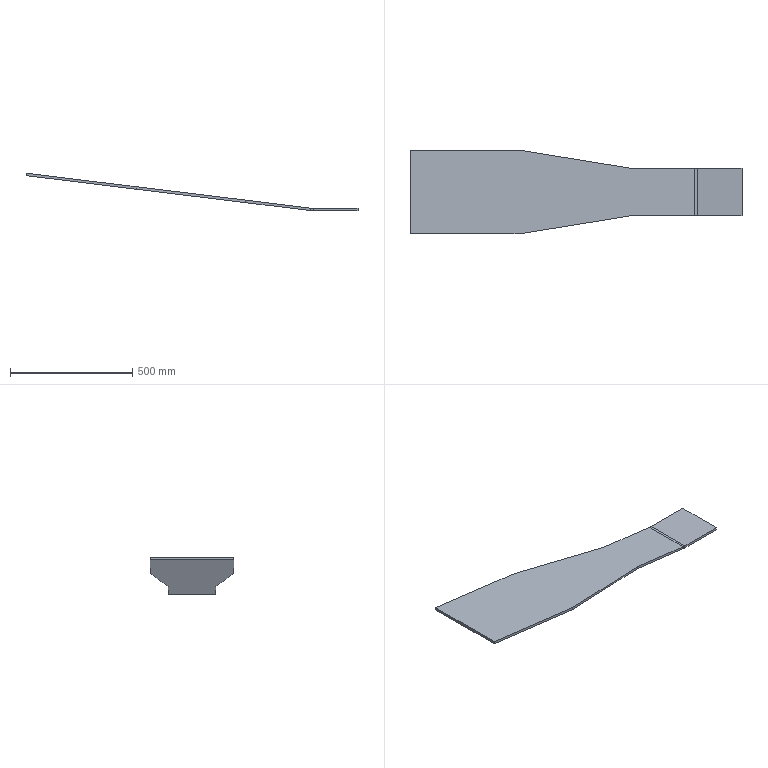Part | SolidWorks | features FlatPattern 1, SM3dBend 1, SMBaseFlange 1, SheetMetal 1 | 1 solid | 18 faces | box 1360 x 340 x 153.769 mm | volume 3656500 mm3 | plane 16 | cylinder 2 | commonest cylinder face diameters 170 x1 190 x1
STEP:
#1=CARTESIAN_POINT('',(1175.139,97.5,0.6336));
#2=VERTEX_POINT('',#1);
#3=CARTESIAN_POINT('',(909.631,97.5,33.234));
#4=VERTEX_POINT('',#3);
#5=CARTESIAN_POINT('',(909.631,97.5,33.234));
#6=DIRECTION('',(-0.9925,0.,0.1219));
#7=VECTOR('',#6,1000.);
#8=LINE('',#5,#7);
#9=EDGE_CURVE('',#2,#4,#8,.T.);
#10=ORIENTED_EDGE('',*,*,#9,.F.);
#11=CARTESIAN_POINT('',(1173.92,97.5,-9.292));
#12=VERTEX_POINT('',#11);
#13=CARTESIAN_POINT('',(1173.92,97.5,-9.292));
#14=DIRECTION('',(-0.1219,0.,-0.9925));
#15=VECTOR('',#14,1000.);
#16=LINE('',#13,#15);
#17=EDGE_CURVE('',#2,#12,#16,.T.);
#18=ORIENTED_EDGE('',*,*,#17,.T.);
#19=CARTESIAN_POINT('',(908.412,97.5,23.308));
#20=VERTEX_POINT('',#19);
#21=CARTESIAN_POINT('',(908.412,97.5,23.308));
#22=DIRECTION('',(-0.9925,0.,0.1219));
#23=VECTOR('',#22,1000.);
#24=LINE('',#21,#23);
#25=EDGE_CURVE('',#12,#20,#24,.T.);
#26=ORIENTED_EDGE('',*,*,#25,.T.);
#27=CARTESIAN_POINT('',(908.412,97.5,23.308));
#28=DIRECTION('',(0.1219,0.,0.9925));
#29=VECTOR('',#28,1000.);
#30=LINE('',#27,#29);
#31=EDGE_CURVE('',#20,#4,#30,.T.);
#32=ORIENTED_EDGE('',*,*,#31,.T.);
#33=EDGE_LOOP('',(#10,#18,#26,#32));
#34=FACE_OUTER_BOUND('',#33,.T.);
#35=CARTESIAN_POINT('',(908.412,97.5,23.308));
#36=DIRECTION('',(0.,1.,0.));
#37=DIRECTION('',(0.1219,0.,0.9925));
#38=AXIS2_PLACEMENT_3D('',#35,#36,#37);
#39=PLANE('',#38);
#40=ADVANCED_FACE('',(#34),#39,.T.);
#41=CARTESIAN_POINT('',(908.412,-97.5,23.308));
#42=VERTEX_POINT('',#41);
#43=CARTESIAN_POINT('',(1173.92,-97.5,-9.292));
#44=VERTEX_POINT('',#43);
#45=CARTESIAN_POINT('',(908.412,-97.5,23.308));
#46=DIRECTION('',(0.9925,0.,-0.1219));
#47=VECTOR('',#46,1000.);
#48=LINE('',#45,#47);
#49=EDGE_CURVE('',#42,#44,#48,.T.);
#50=ORIENTED_EDGE('',*,*,#49,.T.);
#51=CARTESIAN_POINT('',(1175.139,-97.5,0.6336));
#52=VERTEX_POINT('',#51);
#53=CARTESIAN_POINT('',(1173.92,-97.5,-9.292));
#54=DIRECTION('',(0.1219,0.,0.9925));
#55=VECTOR('',#54,1000.);
#56=LINE('',#53,#55);
#57=EDGE_CURVE('',#44,#52,#56,.T.);
#58=ORIENTED_EDGE('',*,*,#57,.T.);
#59=CARTESIAN_POINT('',(909.631,-97.5,33.234));
#60=VERTEX_POINT('',#59);
#61=CARTESIAN_POINT('',(909.631,-97.5,33.234));
#62=DIRECTION('',(0.9925,0.,-0.1219));
#63=VECTOR('',#62,1000.);
#64=LINE('',#61,#63);
#65=EDGE_CURVE('',#60,#52,#64,.T.);
#66=ORIENTED_EDGE('',*,*,#65,.F.);
#67=CARTESIAN_POINT('',(908.412,-97.5,23.308));
#68=DIRECTION('',(0.1219,0.,0.9925));
#69=VECTOR('',#68,1000.);
#70=LINE('',#67,#69);
#71=EDGE_CURVE('',#42,#60,#70,.T.);
#72=ORIENTED_EDGE('',*,*,#71,.F.);
#73=EDGE_LOOP('',(#50,#58,#66,#72));
#74=FACE_OUTER_BOUND('',#73,.T.);
#75=CARTESIAN_POINT('',(908.412,-97.5,23.308));
#76=DIRECTION('',(0.,-1.,0.));
#77=DIRECTION('',(-0.1219,0.,-0.9925));
#78=AXIS2_PLACEMENT_3D('',#75,#76,#77);
#79=PLANE('',#78);
#80=ADVANCED_FACE('',(#74),#79,.T.);
#81=ORIENTED_EDGE('',*,*,#65,.T.);
#82=CARTESIAN_POINT('',(1175.139,-170.,0.6336));
#83=DIRECTION('',(0.,1.,0.));
#84=VECTOR('',#83,1000.);
#85=LINE('',#82,#84);
#86=EDGE_CURVE('',#52,#2,#85,.T.);
#87=ORIENTED_EDGE('',*,*,#86,.T.);
#88=ORIENTED_EDGE('',*,*,#9,.T.);
#89=CARTESIAN_POINT('',(462.985,170.,88.075));
#90=VERTEX_POINT('',#89);
#91=CARTESIAN_POINT('',(462.985,170.,88.075));
#92=DIRECTION('',(-0.9799,0.1591,0.1203));
#93=VECTOR('',#92,1000.);
#94=LINE('',#91,#93);
#95=EDGE_CURVE('',#4,#90,#94,.T.);
#96=ORIENTED_EDGE('',*,*,#95,.T.);
#97=CARTESIAN_POINT('',(9.391,170.,143.769));
#98=VERTEX_POINT('',#97);
#99=CARTESIAN_POINT('',(9.391,170.,143.769));
#100=DIRECTION('',(-0.9925,0.,0.1219));
#101=VECTOR('',#100,1000.);
#102=LINE('',#99,#101);
#103=EDGE_CURVE('',#90,#98,#102,.T.);
#104=ORIENTED_EDGE('',*,*,#103,.T.);
#105=CARTESIAN_POINT('',(9.391,-170.,143.769));
#106=VERTEX_POINT('',#105);
#107=CARTESIAN_POINT('',(9.391,170.,143.769));
#108=DIRECTION('',(0.,-1.,0.));
#109=VECTOR('',#108,1000.);
#110=LINE('',#107,#109);
#111=EDGE_CURVE('',#98,#106,#110,.T.);
#112=ORIENTED_EDGE('',*,*,#111,.T.);
#113=CARTESIAN_POINT('',(462.985,-170.,88.075));
#114=VERTEX_POINT('',#113);
#115=CARTESIAN_POINT('',(9.391,-170.,143.769));
#116=DIRECTION('',(0.9925,0.,-0.1219));
#117=VECTOR('',#116,1000.);
#118=LINE('',#115,#117);
#119=EDGE_CURVE('',#106,#114,#118,.T.);
#120=ORIENTED_EDGE('',*,*,#119,.T.);
#121=CARTESIAN_POINT('',(462.985,-170.,88.075));
#122=DIRECTION('',(0.9799,0.1591,-0.1203));
#123=VECTOR('',#122,1000.);
#124=LINE('',#121,#123);
#125=EDGE_CURVE('',#114,#60,#124,.T.);
#126=ORIENTED_EDGE('',*,*,#125,.T.);
#127=EDGE_LOOP('',(#81,#87,#88,#96,#104,#112,#120,#126));
#128=FACE_OUTER_BOUND('',#127,.T.);
#129=CARTESIAN_POINT('',(1367.194,-170.,-22.948));
#130=DIRECTION('',(0.1219,0.,0.9925));
#131=DIRECTION('',(0.9925,0.,-0.1219));
#132=AXIS2_PLACEMENT_3D('',#129,#130,#131);
#133=PLANE('',#132);
#134=ADVANCED_FACE('',(#128),#133,.T.);
#135=ORIENTED_EDGE('',*,*,#119,.F.);
#136=CARTESIAN_POINT('',(8.173,-170.,133.844));
#137=VERTEX_POINT('',#136);
#138=CARTESIAN_POINT('',(8.173,-170.,133.844));
#139=DIRECTION('',(0.1219,0.,0.9925));
#140=VECTOR('',#139,1000.);
#141=LINE('',#138,#140);
#142=EDGE_CURVE('',#137,#106,#141,.T.);
#143=ORIENTED_EDGE('',*,*,#142,.F.);
#144=CARTESIAN_POINT('',(461.766,-170.,78.15));
#145=VERTEX_POINT('',#144);
#146=CARTESIAN_POINT('',(8.173,-170.,133.844));
#147=DIRECTION('',(0.9925,0.,-0.1219));
#148=VECTOR('',#147,1000.);
#149=LINE('',#146,#148);
#150=EDGE_CURVE('',#137,#145,#149,.T.);
#151=ORIENTED_EDGE('',*,*,#150,.T.);
#152=CARTESIAN_POINT('',(461.766,-170.,78.15));
#153=DIRECTION('',(0.1219,0.,0.9925));
#154=VECTOR('',#153,1000.);
#155=LINE('',#152,#154);
#156=EDGE_CURVE('',#145,#114,#155,.T.);
#157=ORIENTED_EDGE('',*,*,#156,.T.);
#158=EDGE_LOOP('',(#135,#143,#151,#157));
#159=FACE_OUTER_BOUND('',#158,.T.);
#160=CARTESIAN_POINT('',(8.173,-170.,133.844));
#161=DIRECTION('',(0.,-1.,0.));
#162=DIRECTION('',(-0.1219,0.,-0.9925));
#163=AXIS2_PLACEMENT_3D('',#160,#161,#162);
#164=PLANE('',#163);
#165=ADVANCED_FACE('',(#159),#164,.T.);
#166=ORIENTED_EDGE('',*,*,#111,.F.);
#167=CARTESIAN_POINT('',(8.173,170.,133.844));
#168=VERTEX_POINT('',#167);
#169=CARTESIAN_POINT('',(8.173,170.,133.844));
#170=DIRECTION('',(0.1219,0.,0.9925));
#171=VECTOR('',#170,1000.);
#172=LINE('',#169,#171);
#173=EDGE_CURVE('',#168,#98,#172,.T.);
#174=ORIENTED_EDGE('',*,*,#173,.F.);
#175=CARTESIAN_POINT('',(8.173,170.,133.844));
#176=DIRECTION('',(0.,-1.,0.));
#177=VECTOR('',#176,1000.);
#178=LINE('',#175,#177);
#179=EDGE_CURVE('',#168,#137,#178,.T.);
#180=ORIENTED_EDGE('',*,*,#179,.T.);
#181=ORIENTED_EDGE('',*,*,#142,.T.);
#182=EDGE_LOOP('',(#166,#174,#180,#181));
#183=FACE_OUTER_BOUND('',#182,.T.);
#184=CARTESIAN_POINT('',(8.173,170.,133.844));
#185=DIRECTION('',(-0.9925,0.,0.1219));
#186=DIRECTION('',(0.1219,0.,0.9925));
#187=AXIS2_PLACEMENT_3D('',#184,#185,#186);
#188=PLANE('',#187);
#189=ADVANCED_FACE('',(#183),#188,.T.);
#190=ORIENTED_EDGE('',*,*,#103,.F.);
#191=CARTESIAN_POINT('',(461.766,170.,78.15));
#192=VERTEX_POINT('',#191);
#193=CARTESIAN_POINT('',(461.766,170.,78.15));
#194=DIRECTION('',(0.1219,0.,0.9925));
#195=VECTOR('',#194,1000.);
#196=LINE('',#193,#195);
#197=EDGE_CURVE('',#192,#90,#196,.T.);
#198=ORIENTED_EDGE('',*,*,#197,.F.);
#199=CARTESIAN_POINT('',(8.173,170.,133.844));
#200=DIRECTION('',(-0.9925,0.,0.1219));
#201=VECTOR('',#200,1000.);
#202=LINE('',#199,#201);
#203=EDGE_CURVE('',#192,#168,#202,.T.);
#204=ORIENTED_EDGE('',*,*,#203,.T.);
#205=ORIENTED_EDGE('',*,*,#173,.T.);
#206=EDGE_LOOP('',(#190,#198,#204,#205));
#207=FACE_OUTER_BOUND('',#206,.T.);
#208=CARTESIAN_POINT('',(8.173,170.,133.844));
#209=DIRECTION('',(0.,1.,0.));
#210=DIRECTION('',(0.1219,0.,0.9925));
#211=AXIS2_PLACEMENT_3D('',#208,#209,#210);
#212=PLANE('',#211);
#213=ADVANCED_FACE('',(#207),#212,.T.);
#214=ORIENTED_EDGE('',*,*,#95,.F.);
#215=ORIENTED_EDGE('',*,*,#31,.F.);
#216=CARTESIAN_POINT('',(461.766,170.,78.15));
#217=DIRECTION('',(-0.9799,0.1591,0.1203));
#218=VECTOR('',#217,1000.);
#219=LINE('',#216,#218);
#220=EDGE_CURVE('',#20,#192,#219,.T.);
#221=ORIENTED_EDGE('',*,*,#220,.T.);
#222=ORIENTED_EDGE('',*,*,#197,.T.);
#223=EDGE_LOOP('',(#214,#215,#221,#222));
#224=FACE_OUTER_BOUND('',#223,.T.);
#225=CARTESIAN_POINT('',(461.766,170.,78.15));
#226=DIRECTION('',(0.1579,0.9873,-0.01938));
#227=DIRECTION('',(-0.9799,0.1591,0.1203));
#228=AXIS2_PLACEMENT_3D('',#225,#226,#227);
#229=PLANE('',#228);
#230=ADVANCED_FACE('',(#224),#229,.T.);
#231=ORIENTED_EDGE('',*,*,#125,.F.);
#232=ORIENTED_EDGE('',*,*,#156,.F.);
#233=CARTESIAN_POINT('',(461.766,-170.,78.15));
#234=DIRECTION('',(0.9799,0.1591,-0.1203));
#235=VECTOR('',#234,1000.);
#236=LINE('',#233,#235);
#237=EDGE_CURVE('',#145,#42,#236,.T.);
#238=ORIENTED_EDGE('',*,*,#237,.T.);
#239=ORIENTED_EDGE('',*,*,#71,.T.);
#240=EDGE_LOOP('',(#231,#232,#238,#239));
#241=FACE_OUTER_BOUND('',#240,.T.);
#242=CARTESIAN_POINT('',(461.766,-170.,78.15));
#243=DIRECTION('',(0.1579,-0.9873,-0.01938));
#244=DIRECTION('',(0.9799,0.1591,-0.1203));
#245=AXIS2_PLACEMENT_3D('',#242,#243,#244);
#246=PLANE('',#245);
#247=ADVANCED_FACE('',(#241),#246,.T.);
#248=CARTESIAN_POINT('',(1173.92,-170.,-9.292));
#249=DIRECTION('',(0.,1.,0.));
#250=VECTOR('',#249,1000.);
#251=LINE('',#248,#250);
#252=EDGE_CURVE('',#44,#12,#251,.T.);
#253=ORIENTED_EDGE('',*,*,#252,.F.);
#254=ORIENTED_EDGE('',*,*,#49,.F.);
#255=ORIENTED_EDGE('',*,*,#237,.F.);
#256=ORIENTED_EDGE('',*,*,#150,.F.);
#257=ORIENTED_EDGE('',*,*,#179,.F.);
#258=ORIENTED_EDGE('',*,*,#203,.F.);
#259=ORIENTED_EDGE('',*,*,#220,.F.);
#260=ORIENTED_EDGE('',*,*,#25,.F.);
#261=EDGE_LOOP('',(#253,#254,#255,#256,#257,#258,#259,#260));
#262=FACE_OUTER_BOUND('',#261,.T.);
#263=CARTESIAN_POINT('',(1365.976,-170.,-32.873));
#264=DIRECTION('',(0.1219,0.,0.9925));
#265=DIRECTION('',(0.9925,0.,-0.1219));
#266=AXIS2_PLACEMENT_3D('',#263,#264,#265);
#267=PLANE('',#266);
#268=ADVANCED_FACE('',(#262),#267,.F.);
#269=CARTESIAN_POINT('',(1368.,-97.5,0.));
#270=VERTEX_POINT('',#269);
#271=CARTESIAN_POINT('',(1368.,97.5,0.));
#272=VERTEX_POINT('',#271);
#273=CARTESIAN_POINT('',(1368.,-97.5,0.));
#274=DIRECTION('',(0.,1.,0.));
#275=VECTOR('',#274,1000.);
#276=LINE('',#273,#275);
#277=EDGE_CURVE('',#270,#272,#276,.T.);
#278=ORIENTED_EDGE('',*,*,#277,.F.);
#279=CARTESIAN_POINT('',(1368.,-97.5,-10.));
#280=VERTEX_POINT('',#279);
#281=CARTESIAN_POINT('',(1368.,-97.5,-10.));
#282=DIRECTION('',(0.,0.,1.));
#283=VECTOR('',#282,1000.);
#284=LINE('',#281,#283);
#285=EDGE_CURVE('',#280,#270,#284,.T.);
#286=ORIENTED_EDGE('',*,*,#285,.F.);
#287=CARTESIAN_POINT('',(1368.,97.5,-10.));
#288=VERTEX_POINT('',#287);
#289=CARTESIAN_POINT('',(1368.,-97.5,-10.));
#290=DIRECTION('',(0.,1.,0.));
#291=VECTOR('',#290,1000.);
#292=LINE('',#289,#291);
#293=EDGE_CURVE('',#280,#288,#292,.T.);
#294=ORIENTED_EDGE('',*,*,#293,.T.);
#295=CARTESIAN_POINT('',(1368.,97.5,-10.));
#296=DIRECTION('',(0.,0.,1.));
#297=VECTOR('',#296,1000.);
#298=LINE('',#295,#297);
#299=EDGE_CURVE('',#288,#272,#298,.T.);
#300=ORIENTED_EDGE('',*,*,#299,.T.);
#301=EDGE_LOOP('',(#278,#286,#294,#300));
#302=FACE_OUTER_BOUND('',#301,.T.);
#303=CARTESIAN_POINT('',(1368.,-97.5,-10.));
#304=DIRECTION('',(1.,0.,0.));
#305=DIRECTION('',(0.,0.,-1.));
#306=AXIS2_PLACEMENT_3D('',#303,#304,#305);
#307=PLANE('',#306);
#308=ADVANCED_FACE('',(#302),#307,.T.);
#309=CARTESIAN_POINT('',(1185.498,-97.5,-10.));
#310=VERTEX_POINT('',#309);
#311=CARTESIAN_POINT('',(907.,-97.5,-10.));
#312=DIRECTION('',(1.,0.,0.));
#313=VECTOR('',#312,1000.);
#314=LINE('',#311,#313);
#315=EDGE_CURVE('',#310,#280,#314,.T.);
#316=ORIENTED_EDGE('',*,*,#315,.F.);
#317=CARTESIAN_POINT('',(1185.498,97.5,-10.));
#318=VERTEX_POINT('',#317);
#319=CARTESIAN_POINT('',(1185.498,-170.,-10.));
#320=DIRECTION('',(0.,1.,0.));
#321=VECTOR('',#320,1000.);
#322=LINE('',#319,#321);
#323=EDGE_CURVE('',#310,#318,#322,.T.);
#324=ORIENTED_EDGE('',*,*,#323,.T.);
#325=CARTESIAN_POINT('',(907.,97.5,-10.));
#326=DIRECTION('',(-1.,0.,0.));
#327=VECTOR('',#326,1000.);
#328=LINE('',#325,#327);
#329=EDGE_CURVE('',#288,#318,#328,.T.);
#330=ORIENTED_EDGE('',*,*,#329,.F.);
#331=ORIENTED_EDGE('',*,*,#293,.F.);
#332=EDGE_LOOP('',(#316,#324,#330,#331));
#333=FACE_OUTER_BOUND('',#332,.T.);
#334=CARTESIAN_POINT('',(1368.,-170.,-10.));
#335=DIRECTION('',(0.,0.,1.));
#336=DIRECTION('',(1.,0.,0.));
#337=AXIS2_PLACEMENT_3D('',#334,#335,#336);
#338=PLANE('',#337);
#339=ADVANCED_FACE('',(#333),#338,.F.);
#340=CARTESIAN_POINT('',(1185.498,97.5,0.));
#341=VERTEX_POINT('',#340);
#342=CARTESIAN_POINT('',(1185.498,97.5,-10.));
#343=DIRECTION('',(0.,0.,-1.));
#344=VECTOR('',#343,1000.);
#345=LINE('',#342,#344);
#346=EDGE_CURVE('',#341,#318,#345,.T.);
#347=ORIENTED_EDGE('',*,*,#346,.F.);
#348=CARTESIAN_POINT('',(907.,97.5,0.));
#349=DIRECTION('',(-1.,0.,0.));
#350=VECTOR('',#349,1000.);
#351=LINE('',#348,#350);
#352=EDGE_CURVE('',#272,#341,#351,.T.);
#353=ORIENTED_EDGE('',*,*,#352,.F.);
#354=ORIENTED_EDGE('',*,*,#299,.F.);
#355=ORIENTED_EDGE('',*,*,#329,.T.);
#356=EDGE_LOOP('',(#347,#353,#354,#355));
#357=FACE_OUTER_BOUND('',#356,.T.);
#358=CARTESIAN_POINT('',(907.,97.5,-10.));
#359=DIRECTION('',(0.,1.,0.));
#360=DIRECTION('',(0.,0.,1.));
#361=AXIS2_PLACEMENT_3D('',#358,#359,#360);
#362=PLANE('',#361);
#363=ADVANCED_FACE('',(#357),#362,.T.);
#364=CARTESIAN_POINT('',(1185.498,-97.5,0.));
#365=VERTEX_POINT('',#364);
#366=CARTESIAN_POINT('',(1185.498,-170.,0.));
#367=DIRECTION('',(0.,1.,0.));
#368=VECTOR('',#367,1000.);
#369=LINE('',#366,#368);
#370=EDGE_CURVE('',#365,#341,#369,.T.);
#371=ORIENTED_EDGE('',*,*,#370,.F.);
#372=CARTESIAN_POINT('',(907.,-97.5,0.));
#373=DIRECTION('',(1.,0.,0.));
#374=VECTOR('',#373,1000.);
#375=LINE('',#372,#374);
#376=EDGE_CURVE('',#365,#270,#375,.T.);
#377=ORIENTED_EDGE('',*,*,#376,.T.);
#378=ORIENTED_EDGE('',*,*,#277,.T.);
#379=ORIENTED_EDGE('',*,*,#352,.T.);
#380=EDGE_LOOP('',(#371,#377,#378,#379));
#381=FACE_OUTER_BOUND('',#380,.T.);
#382=CARTESIAN_POINT('',(1368.,-170.,0.));
#383=DIRECTION('',(0.,0.,1.));
#384=DIRECTION('',(1.,0.,0.));
#385=AXIS2_PLACEMENT_3D('',#382,#383,#384);
#386=PLANE('',#385);
#387=ADVANCED_FACE('',(#381),#386,.T.);
#388=CARTESIAN_POINT('',(1185.498,-97.5,-10.));
#389=DIRECTION('',(0.,0.,1.));
#390=VECTOR('',#389,1000.);
#391=LINE('',#388,#390);
#392=EDGE_CURVE('',#310,#365,#391,.T.);
#393=ORIENTED_EDGE('',*,*,#392,.F.);
#394=ORIENTED_EDGE('',*,*,#315,.T.);
#395=ORIENTED_EDGE('',*,*,#285,.T.);
#396=ORIENTED_EDGE('',*,*,#376,.F.);
#397=EDGE_LOOP('',(#393,#394,#395,#396));
#398=FACE_OUTER_BOUND('',#397,.T.);
#399=CARTESIAN_POINT('',(907.,-97.5,-10.));
#400=DIRECTION('',(0.,-1.,0.));
#401=DIRECTION('',(0.,0.,-1.));
#402=AXIS2_PLACEMENT_3D('',#399,#400,#401);
#403=PLANE('',#402);
#404=ADVANCED_FACE('',(#398),#403,.T.);
#405=ORIENTED_EDGE('',*,*,#392,.T.);
#406=CARTESIAN_POINT('',(1185.498,-97.5,85.));
#407=DIRECTION('',(0.,1.,0.));
#408=DIRECTION('',(0.,0.,1.));
#409=AXIS2_PLACEMENT_3D('',#406,#407,#408);
#410=CIRCLE('',#409,85.);
#411=EDGE_CURVE('',#365,#52,#410,.T.);
#412=ORIENTED_EDGE('',*,*,#411,.T.);
#413=ORIENTED_EDGE('',*,*,#57,.F.);
#414=CARTESIAN_POINT('',(1185.498,-97.5,85.));
#415=DIRECTION('',(0.,1.,0.));
#416=DIRECTION('',(0.,0.,-1.));
#417=AXIS2_PLACEMENT_3D('',#414,#415,#416);
#418=CIRCLE('',#417,95.);
#419=EDGE_CURVE('',#310,#44,#418,.T.);
#420=ORIENTED_EDGE('',*,*,#419,.F.);
#421=EDGE_LOOP('',(#405,#412,#413,#420));
#422=FACE_OUTER_BOUND('',#421,.T.);
#423=CARTESIAN_POINT('',(1185.498,-97.5,85.));
#424=DIRECTION('',(0.,-1.,0.));
#425=DIRECTION('',(0.,0.,-1.));
#426=AXIS2_PLACEMENT_3D('',#423,#424,#425);
#427=PLANE('',#426);
#428=ADVANCED_FACE('',(#422),#427,.T.);
#429=ORIENTED_EDGE('',*,*,#17,.F.);
#430=CARTESIAN_POINT('',(1185.498,97.5,85.));
#431=DIRECTION('',(0.,-1.,0.));
#432=DIRECTION('',(0.,0.,1.));
#433=AXIS2_PLACEMENT_3D('',#430,#431,#432);
#434=CIRCLE('',#433,85.);
#435=EDGE_CURVE('',#2,#341,#434,.T.);
#436=ORIENTED_EDGE('',*,*,#435,.T.);
#437=ORIENTED_EDGE('',*,*,#346,.T.);
#438=CARTESIAN_POINT('',(1185.498,97.5,85.));
#439=DIRECTION('',(0.,-1.,0.));
#440=DIRECTION('',(0.,0.,1.));
#441=AXIS2_PLACEMENT_3D('',#438,#439,#440);
#442=CIRCLE('',#441,95.);
#443=EDGE_CURVE('',#12,#318,#442,.T.);
#444=ORIENTED_EDGE('',*,*,#443,.F.);
#445=EDGE_LOOP('',(#429,#436,#437,#444));
#446=FACE_OUTER_BOUND('',#445,.T.);
#447=CARTESIAN_POINT('',(1185.498,97.5,85.));
#448=DIRECTION('',(0.,1.,0.));
#449=DIRECTION('',(0.,0.,1.));
#450=AXIS2_PLACEMENT_3D('',#447,#448,#449);
#451=PLANE('',#450);
#452=ADVANCED_FACE('',(#446),#451,.T.);
#453=ORIENTED_EDGE('',*,*,#443,.T.);
#454=ORIENTED_EDGE('',*,*,#323,.F.);
#455=ORIENTED_EDGE('',*,*,#419,.T.);
#456=ORIENTED_EDGE('',*,*,#252,.T.);
#457=EDGE_LOOP('',(#453,#454,#455,#456));
#458=FACE_OUTER_BOUND('',#457,.T.);
#459=CARTESIAN_POINT('',(1185.498,-195.566,85.));
#460=DIRECTION('',(0.,1.,0.));
#461=DIRECTION('',(0.,0.,1.));
#462=AXIS2_PLACEMENT_3D('',#459,#460,#461);
#463=CYLINDRICAL_SURFACE('',#462,95.);
#464=ADVANCED_FACE('',(#458),#463,.T.);
#465=ORIENTED_EDGE('',*,*,#435,.F.);
#466=ORIENTED_EDGE('',*,*,#86,.F.);
#467=ORIENTED_EDGE('',*,*,#411,.F.);
#468=ORIENTED_EDGE('',*,*,#370,.T.);
#469=EDGE_LOOP('',(#465,#466,#467,#468));
#470=FACE_OUTER_BOUND('',#469,.T.);
#471=CARTESIAN_POINT('',(1185.498,-195.566,85.));
#472=DIRECTION('',(0.,1.,0.));
#473=DIRECTION('',(0.,0.,1.));
#474=AXIS2_PLACEMENT_3D('',#471,#472,#473);
#475=CYLINDRICAL_SURFACE('',#474,85.);
#476=ADVANCED_FACE('',(#470),#475,.F.);
#477=CLOSED_SHELL('',(#40,#80,#134,#165,#189,#213,#230,#247,#268,#308,#339,#363,#387,#404,#428,#452,#464,#476));
#478=MANIFOLD_SOLID_BREP('',#477);
#479=CARTESIAN_POINT('',(0.,0.,0.));
#480=DIRECTION('',(0.,0.,1.));
#481=DIRECTION('',(1.,0.,0.));
#482=AXIS2_PLACEMENT_3D('',#479,#480,#481);
#483=(LENGTH_UNIT()NAMED_UNIT(*)SI_UNIT(.MILLI.,.METRE.));
#484=UNCERTAINTY_MEASURE_WITH_UNIT(LENGTH_MEASURE(0.00001),#483,'','');
#485=(NAMED_UNIT(*)PLANE_ANGLE_UNIT()SI_UNIT($,.RADIAN.));
#486=(NAMED_UNIT(*)SI_UNIT($,.STERADIAN.)SOLID_ANGLE_UNIT());
#487=(GEOMETRIC_REPRESENTATION_CONTEXT(3)GLOBAL_UNCERTAINTY_ASSIGNED_CONTEXT((#484))GLOBAL_UNIT_ASSIGNED_CONTEXT((#483,#485,#486))REPRESENTATION_CONTEXT('',''));
#488=ADVANCED_BREP_SHAPE_REPRESENTATION('',(#478,#482),#487);